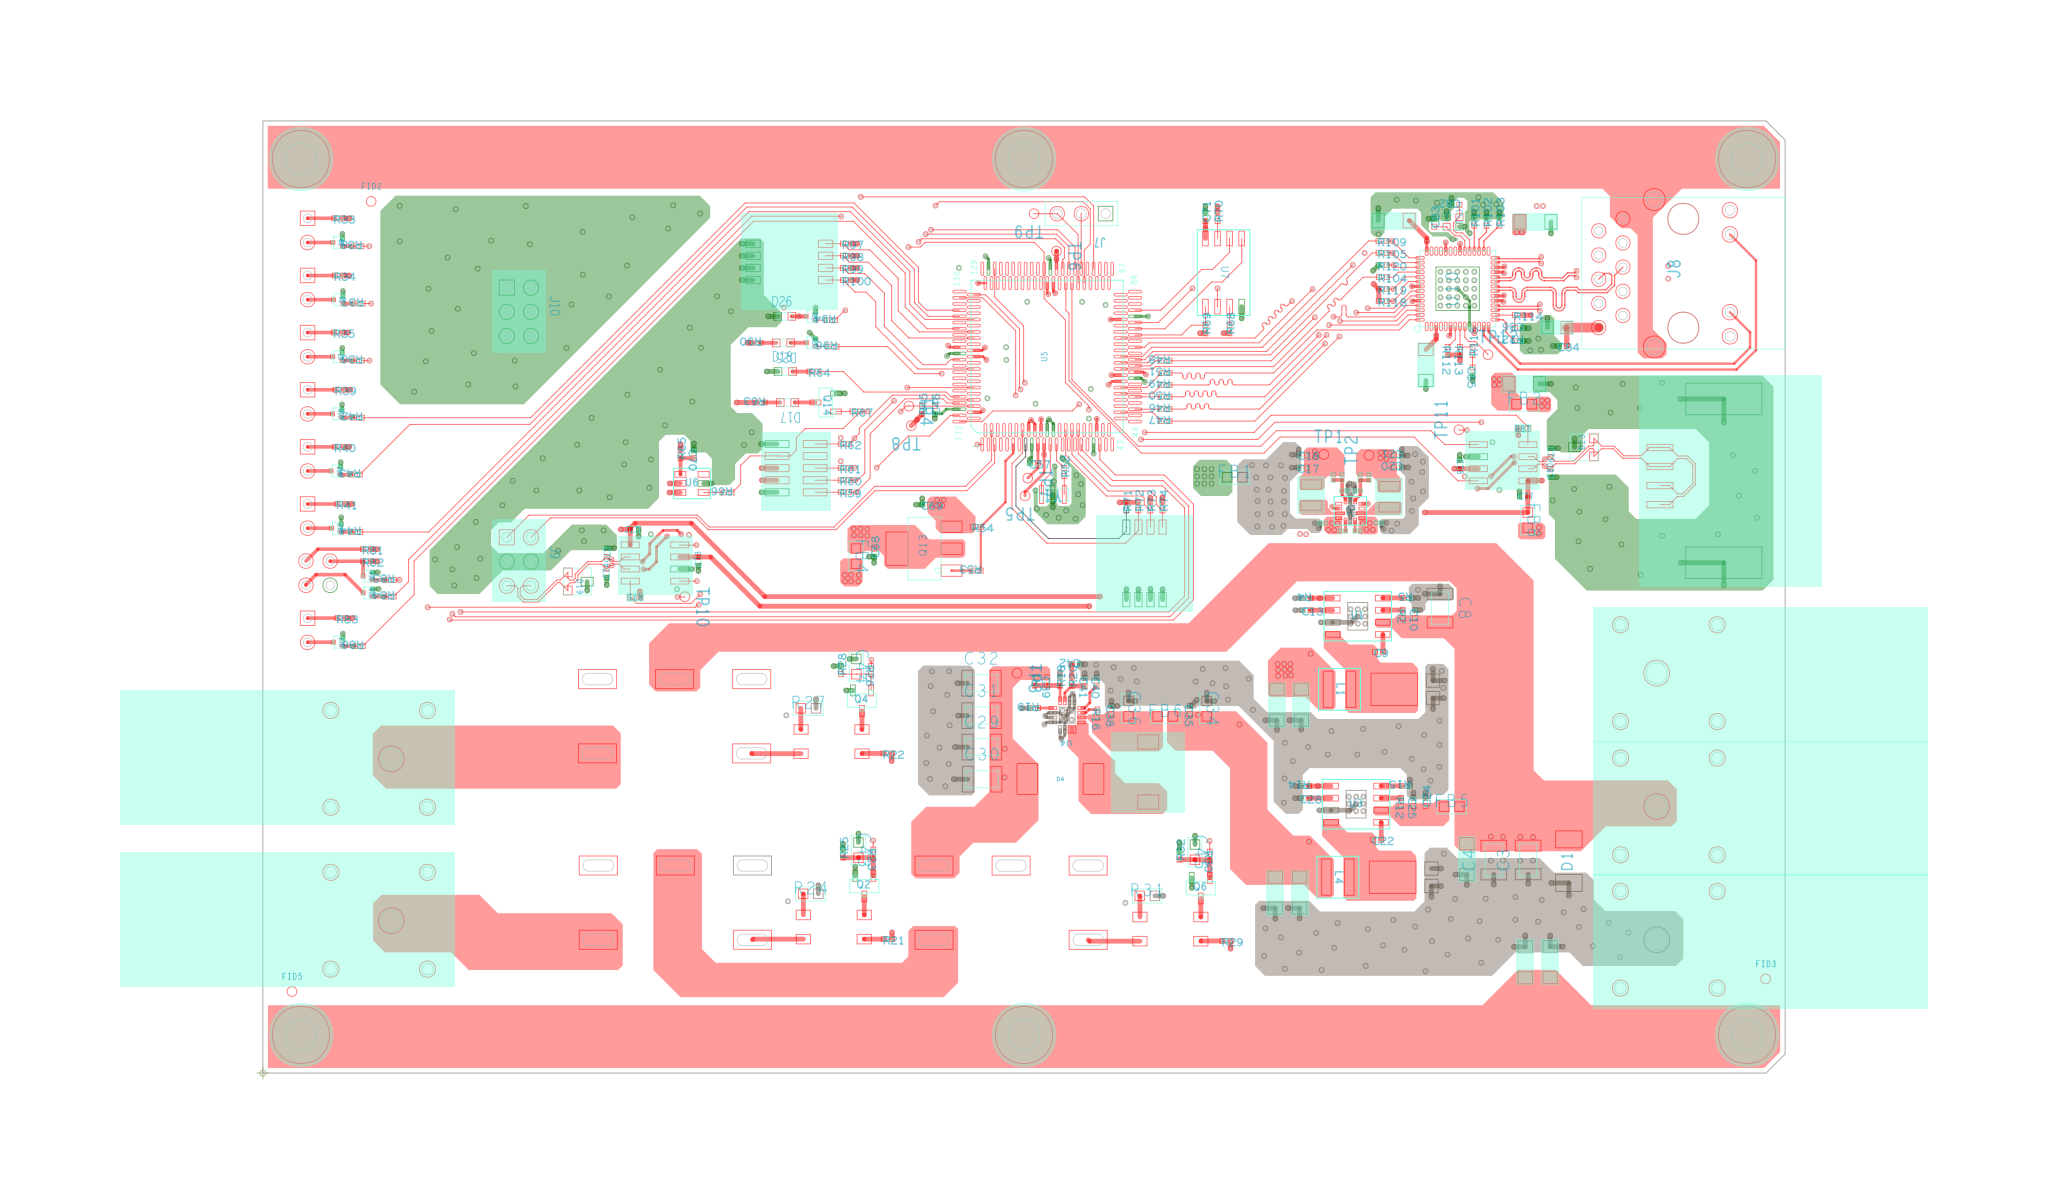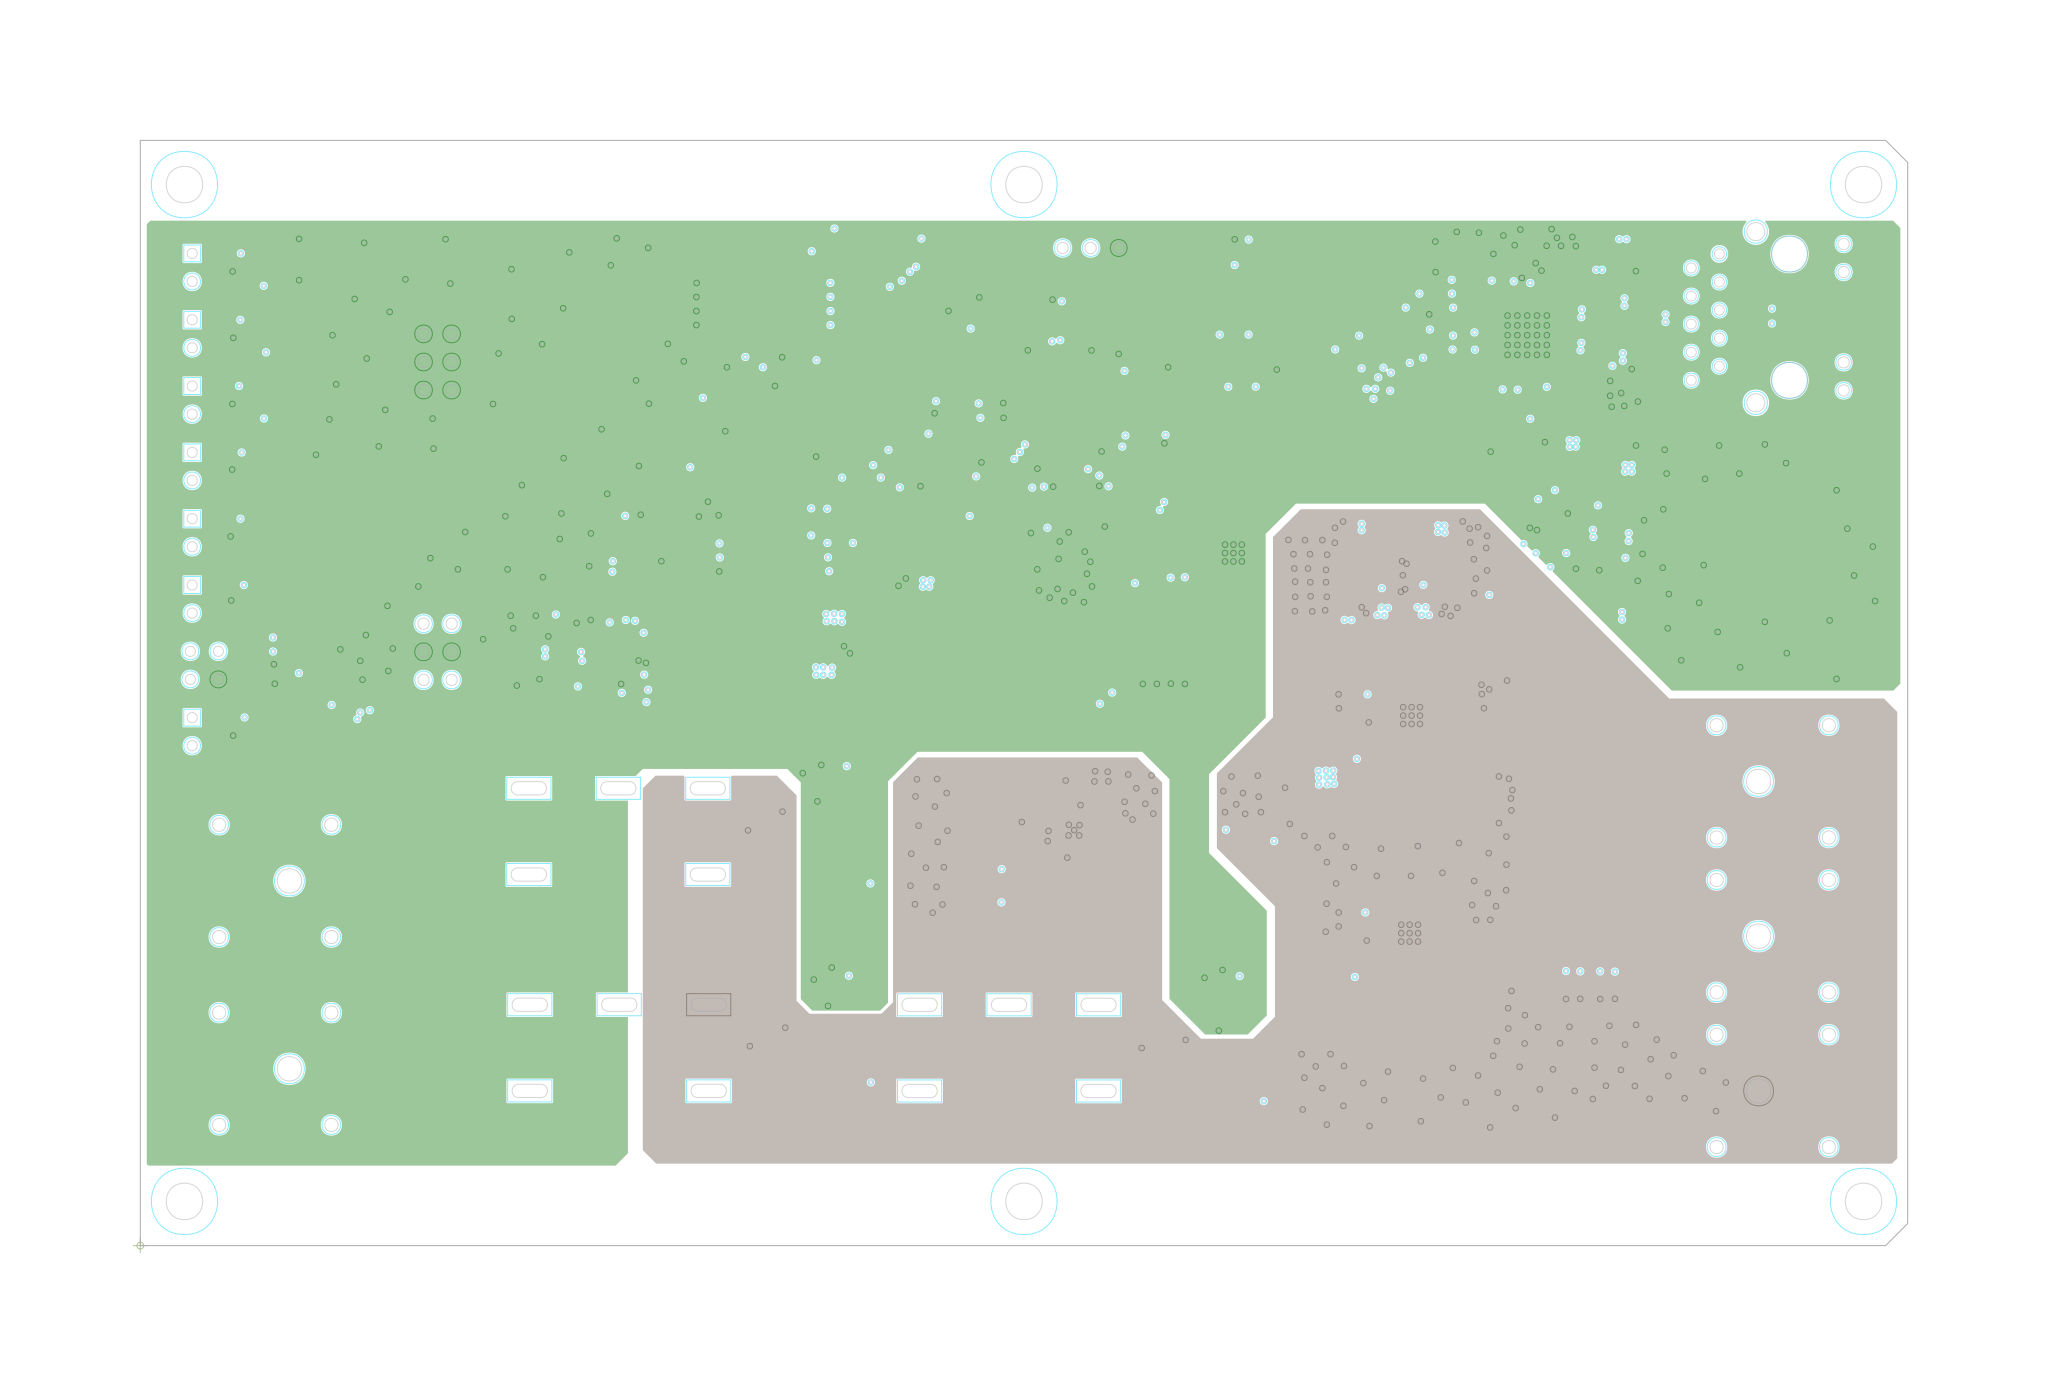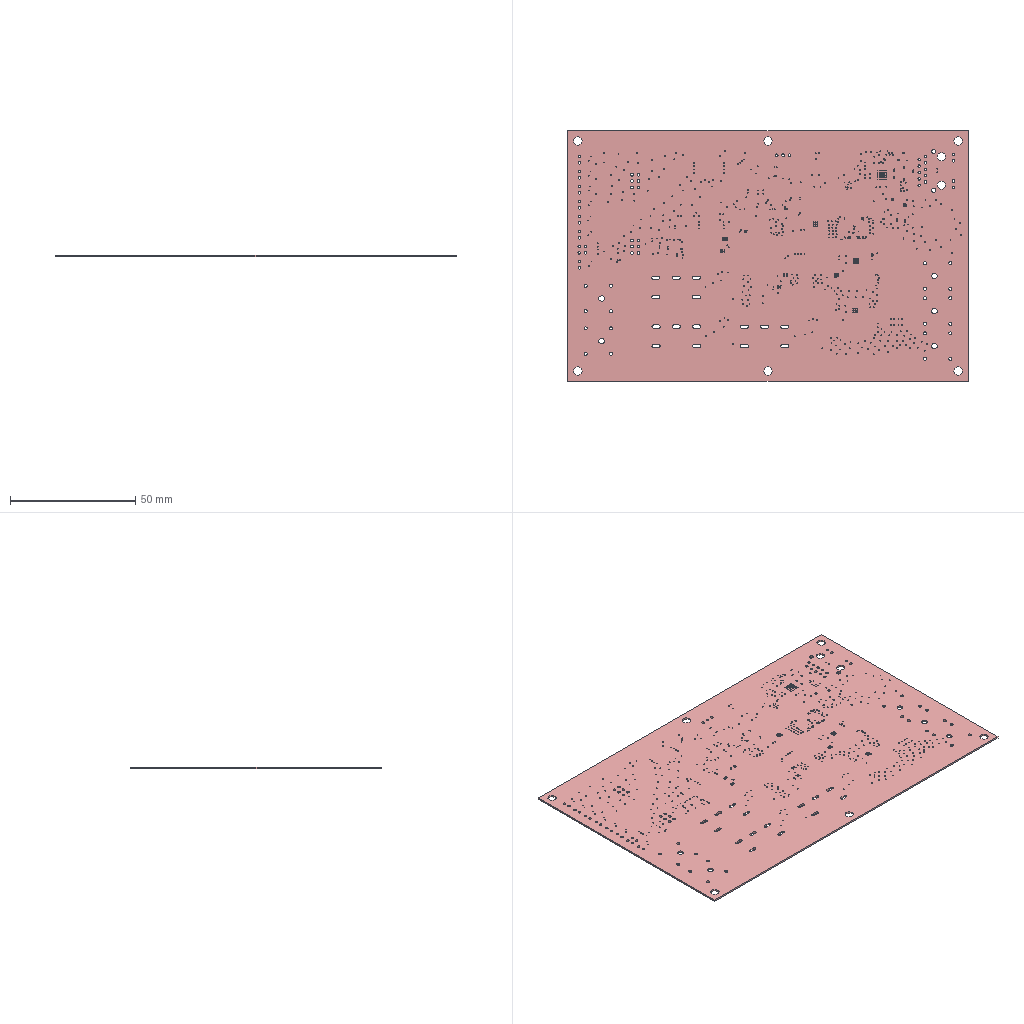Circuit board layout | Cadence Allegro | box 160 x 100 x 0.7 mm
Layer stack:
# Cadence Allegro layer stack of 2 (unit mm; from the constraint file cross-section; dielectric type: 0 not recorded (Allegro does not mark core vs prepreg), 3 surface material)
index,name,kind,layer,copper_thickness_mm,dielectric_type,dielectric_thickness_mm,dielectric_material,dielectric_constant
0,Top Surface,other,,,,,,
1,TOP,copper,TOP,0.0305,,,,
2,Dielectric1,dielectric,,,0,0.2032,FR-4,4.5
3,GND,copper,GND,0.0305,,,,
4,Dielectric2,dielectric,,,0,0.2032,FR-4,4.5
5,POWER,copper,POWER,0.0305,,,,
6,Dielectric3,dielectric,,,0,0.2032,FR-4,4.5
7,BOTTOM,copper,BOTTOM,0.0305,,,,
8,Bottom Surface,other,,,,,,
# drill layer pairs: low layer,high layer
drill_pair,TOP,BOTTOM
Part placement:
REFDES,COMP_VALUE,SYM_NAME,SYM_X,SYM_Y,SYM_ROTATE,SYM_MIRROR
C1,0.1uF,0402,5255.815,929.472,90.000,YES
C2,1nF,0402,5203.236,928.917,270.000,YES
C3,10uF_50V,1210,5236.091,881.236,90.000,NO
C4,10uF_50V,1210,5093.579,880.543,90.000,NO
C5,0.1uF,0402,5132.177,928.886,270.000,YES
C6,0.1uF,0402,5081.394,928.713,270.000,YES
C7,1nF_2kv,1206,5223.642,458.039,270.000,NO
C8,4.7uF_50V,1210,4871.276,1922.413,270.000,NO
C9,0.1uF,0402,4618.441,1741.791,0.000,NO
C10,0.1uF,0402,4768.024,1897.736,270.000,NO
C11,100uF_6.3V,1206,4196.335,1522.984,270.000,NO
C12,100uF_6.3V,1206,4296.965,1523.051,270.000,NO
C13,470pF,0402,4319.169,1913.894,0.000,NO
C14,4.7uF_6.3V,0201,4617.413,2275.484,180.000,NO
C15,4.7uF_6.3V,0201,4386.961,2273.791,0.000,NO
C16,10pF,0201,4431.000,2463.535,90.000,NO
C17,22uF_6.3V,0402,4302.398,2503.622,0.000,NO
C18,22uF_6.3V,0402,4303.248,2556.858,0.000,NO
C19,10pF,0201,4541.429,2462.433,90.000,NO
C20,10uF_6.3V,0402,4696.803,2504.610,180.000,NO
C21,10uF_6.3V,0402,4696.776,2553.764,180.000,NO
C22,0.1uF,0402,4611.441,964.791,0.000,NO
C23,10uF_50V,1206,4982.193,884.799,90.000,NO
C24,1uF,0402,4811.551,1120.925,90.000,NO
C25,0.1uF,0402,4761.024,1120.736,270.000,NO
C26,100uF_6.3V,1206,4289.965,746.051,270.000,NO
C27,100uF_6.3V,1206,4189.335,745.984,270.000,NO
C28,470pF,0402,4312.169,1136.894,0.000,NO
C29,4.7uF_50V,1210,2975.161,1347.945,0.000,NO
C30,4.7uF_50V,1210,2976.256,1215.130,0.000,NO
C31,4.7uF_50V,1210,2974.024,1478.004,0.000,NO
C32,4.7uF_50V,1210,2973.433,1612.031,0.000,NO
C33,10uF_50V,1206,2970.370,1340.913,180.000,YES
C34,10uF_16V,0603,3905.988,1506.535,270.000,NO
C35,0.1uF,0402,3836.575,1501.610,270.000,NO
C36,10uF_16V,0603,3582.047,1507.114,270.000,NO
C37,10uF_50V,1206,2970.870,1222.839,180.000,YES
C38,0.1uF,0402,3511.059,1501.157,270.000,NO
C39,20pF_25V,0402,3245.874,1619.213,270.000,NO
C40,47nF_10V,0402,3450.453,1618.110,270.000,NO
C41,100pF_16V,0402,3400.661,1617.000,270.000,NO
C42,0.1uF,0402,3364.358,1689.886,180.000,NO
C43,2.2nF_50V,0603,2464.520,921.850,270.000,NO
C44,2.2nF_50V,0603,2455.957,1680.697,270.000,NO
C45,2.2nF_50V,0603,3857.189,913.346,270.000,NO
C46,0.1uF,0402,2780.705,2741.437,90.000,NO
C47,10uF_10V,0603,3317.331,3188.803,0.000,YES
C48,0.1uF,0402,3254.417,3266.378,180.000,YES
C49,0.1uF,0402,3549.661,2869.283,270.000,YES
C50,0.1uF,0402,3217.000,2599.795,180.000,YES
C51,0.1uF,0402,3034.114,3001.382,0.000,YES
C52,0.1uF,0402,3236.941,2658.358,0.000,YES
C53,0.1uF,0402,3609.000,2882.224,270.000,YES
C54,0.1uF,0402,3267.819,3325.811,180.000,YES
C55,0.1uF,0402,2882.472,2985.067,270.000,YES
C56,10uF_10V,0603,2794.520,2984.303,270.000,YES
C57,0.22uF,0402,3190.701,2521.654,0.000,NO
C58,10uF_10V,0603,2925.579,3297.961,90.000,YES
C59,0.1uF,0402,3169.465,2751.110,90.000,YES
C60,0.1uF,0402,3033.862,2948.642,0.000,YES
C61,0.1uF,0402,2990.244,3282.819,90.000,YES
C62,0.1uF,0402,3547.087,3132.346,90.000,YES
C63,0.1uF,0402,3442.697,2846.890,180.000,YES
C64,0.1uF,0402,3486.980,3132.303,90.000,YES
C65,0.1uF,0402,3434.421,2658.268,180.000,YES
C66,0.1uF,0402,3211.118,3189.185,180.000,YES
C67,0.1uF,0402,2941.248,2748.118,90.000,YES
C68,2.2uF,0402,2529.287,2151.634,90.000,NO
C69,2.2uF,0402,2744.913,2350.260,0.000,NO
C70,NC,0402,1783.713,2559.197,270.000,NO
C71,0.1uF,0402,3900.539,3539.610,90.000,NO
C72,0.1uF/50V,C0402,1537.614,2249.240,180.000,NO
C73,0.1uF/50V,C0402,1802.283,2116.236,90.000,NO
C74,47pF/50V,C0402,1422.764,2066.839,90.000,NO
C75,47pF/50V,C0402,1422.772,2152.642,270.000,NO
C76,47nF/50V,C0402,1655.654,2196.618,180.000,YES
C77,0.1uF/50V,C0402,5217.319,2383.724,0.000,NO
C78,0.1uF/50V,C0402,4952.650,2516.728,270.000,NO
C79,47pF/50V,C0402,5328.169,2566.126,270.000,NO
C80,47pF/50V,C0402,5329.161,2481.323,90.000,NO
C81,47nF/50V,C0402,5099.280,2436.346,0.000,YES
C82,6pF_1%,0402,4935.124,3590.128,180.000,NO
C83,6pF_1%,0402,4846.808,3515.924,90.000,NO
C84,0.1uF,0402,5379.007,3006.491,0.000,NO
C85,47pF,0402,5006.083,2900.662,270.000,NO
C86,0.1uF,0402,5197.268,3080.205,180.000,NO
C87,0.1uF,0402,4814.862,3388.890,90.000,YES
C88,0.1uF,0402,4914.433,3103.504,270.000,YES
C89,0.1uF,0402,5082.740,3298.197,0.000,YES
C90,0.1uF,0402,5083.543,3232.583,0.000,YES
C91,0.1uF,0402,5013.547,3103.697,270.000,YES
C92,0.1uF,0402,4804.024,3252.988,180.000,YES
C93,0.1uF,0402,4805.969,3191.358,180.000,YES
C94,0.1uF,0402,4902.161,3388.575,90.000,YES
C95,0.1uF,0402,4953.748,3388.339,90.000,YES
C96,0.1uF,0402,5084.028,3182.937,0.000,YES
C97,0.1uF,0402,5083.260,3346.500,0.000,YES
C98,0.1uF,0402,4855.610,3104.161,270.000,YES
CB1,22uF_10V,0805,5355.680,3082.448,180.000,NO
CB2,22uF_10V,1206,4679.571,3525.020,180.000,NO
CB3,22uF_10V,1206,5266.339,3519.437,0.000,NO
CB4,22uF_10V,1206,5219.425,2850.093,0.000,NO
CB5,22uF_10V,1206,4812.812,2927.908,270.000,NO
D1,SMBJ33CA,DO-214AA,5404.406,876.315,90.000,NO
D2,PDS760-13,PDS760,4762.260,1586.618,0.000,NO
D3,PDS760-13,PDS760,4755.260,809.618,0.000,NO
D4,B540C-13-F,SMC,3300.154,1215.972,0.000,NO
D5,SMAJ16A,DO-214AC,2230.827,631.843,90.000,YES
D6,SMAJ16A,DO-214AC,1750.311,552.874,0.000,YES
D7,SMAJ16A,DO-214AC,2220.673,1400.406,90.000,YES
D8,SMAJ16A,DO-214AC,1740.748,1321.720,0.000,YES
D9,SMAJ16A,DO-214AC,3628.323,625.173,90.000,YES
D10,SMAJ16A,DO-214AC,3120.980,550.370,0.000,YES
D11,MHK1375CGBTD,LED-TH_MHK1375CRBTD,185.043,3484.280,270.000,NO
D12,MHK1375CGBTD,LED-TH_MHK1375CRBTD,185.043,3248.059,270.000,NO
D13,MHK1375CGBTD,LED-TH_MHK1375CRBTD,185.043,3011.839,270.000,NO
D14,MHK1375CRBTD,LED-TH_MHK1375CRBTD,185.043,2775.618,270.000,NO
D15,MHK1375CRBTD,LED-TH_MHK1375CRBTD,185.043,2539.398,270.000,NO
D16,MHK1375CRBTD,LED-TH_MHK1375CRBTD,185.043,2303.177,270.000,NO
D17,XL-TD1608SURC,LED0603,2170.984,2772.713,180.000,NO
D18,XL-TD1608SYGC,LED0603,2161.807,2900.945,0.000,NO
D19,SM24CANA-02HTG,SOT23-3,1262.067,2070.106,270.000,NO
D20,CSD87502Q2,DFN-6_2X2,1634.961,2108.839,90.000,YES
D21,MHK2396YGBTD,LED_D3_WX2,228.350,2066.957,270.000,NO
D22,MHK1375CGBTD,LED-TH_MHK1375CRBTD,185.039,1830.709,270.000,NO
D23,SM24CANA-02HTG,SOT23-3,5508.000,2549.929,90.000,NO
D24,CSD87502Q2,DFN-6_2X2,5119.972,2524.126,270.000,YES
D25,XL-TD1608SYGC,LED0603,2154.189,3019.417,180.000,NO
D26,XL-TD1608SURC,LED0603,2159.248,3128.795,0.000,NO
FB1,BLM18KG300TN1D,0603,4022.043,2463.720,0.000,NO
FB2,BLM18KG300TN1D,0603,5219.364,2765.824,0.000,NO
FB3,BLM18KG300TN1D,0603,5234.535,3520.157,180.000,YES
FB4,BLM18KG300TN1D,0603,2454.500,2137.295,270.000,NO
FB5,BLM18KG300TN1D,0603,4919.642,1101.654,0.000,NO
FB6,BLM18KG300TN1D,0603,3734.146,1474.689,0.000,NO
FB7,BLM18KG300TN1D,0603,4367.000,2183.000,0.000,YES
FB8,BLM18KG300TN1D,0603,5234.536,2286.306,270.000,NO
FID1,FIDUCIAL_1MM,MARK40,6218.539,389.295,0.000,YES
FID2,FIDUCIAL_1MM,MARK40,447.854,3604.295,0.000,NO
FID3,FIDUCIAL_1MM,MARK40,6218.657,389.295,0.000,NO
FID4,FIDUCIAL_1MM,MARK40,447.953,3604.295,0.000,YES
FID5,FIDUCIAL_1MM,MARK40,120.244,337.295,0.000,NO
FID6,FIDUCIAL_1MM,MARK40,120.559,337.295,0.000,YES
J1,24.245.2,C7437326,5767.717,1102.362,180.000,NO
J2,24.245.1,C7437326,5767.717,551.181,180.000,NO
J3,24.245.1,C7437326,531.496,1299.213,0.000,NO
J4,24.245.2,C7437326,531.496,629.921,0.000,NO
J5,24.245.1,C7437326,5767.717,1653.543,180.000,NO
J6,Header_JTAG_2x5_1P27mm,JTAG_2X5_1P27MM,2206.571,2501.346,90.000,NO
J7,header_2.54_3,HDR_1X3,3487.157,3553.693,180.000,NO
J8,HR915330AE,HR915330AE,5877.953,3307.087,90.000,NO
J9,A2541WR-2x3P,DIP_2X3_254MM,1059.606,2115.150,270.000,NO
J10,A2541WR-2x3P,DIP_2X3_254MM,1059.606,3147.606,270.000,NO
J11,349128040,349128040,5913.386,2448.819,90.000,NO
L1,FEXL0430A-2R2M,L_41X41_H210_BOURNS,4455.374,1586.843,270.000,NO
L2,DFE252012PD-R47M,1008,4338.772,2389.969,90.000,NO
L3,DFE252012PD-R47M,1008,4661.961,2383.071,90.000,NO
L4,FEXL0430A-2R2M,L_41X41_H210_BOURNS,4448.374,809.843,270.000,NO
L5,SLF7045T100M,SMD_7X7,3663.744,1245.185,270.000,NO
MH1,MOUNTING_HOLE,HOLE3_3MM_6,6141.732,3779.528,0.000,NO
MH2,MOUNTING_HOLE,HOLE3_3MM_6,157.480,3779.528,0.000,NO
MH3,MOUNTING_HOLE,HOLE3_3MM_6,157.480,157.480,0.000,NO
MH4,MOUNTING_HOLE,HOLE3_3MM_6,6141.732,157.480,0.000,NO
MH5,MOUNTING_HOLE,HOLE3_3MM_6,3149.606,157.480,0.000,NO
MH6,MOUNTING_HOLE,HOLE3_3MM_6,3149.606,3779.528,0.000,NO
Q1,TLP187,TLP187,2362.610,603.874,90.000,NO
Q2,BSS138,003_SOT23B,2526.213,815.496,270.000,NO
Q3,TLP187,TLP187,2353.047,1370.720,90.000,NO
Q4,BSS138,003_SOT23B,2516.650,1582.343,270.000,NO
Q5,TLP187,TLP187,3755.280,595.370,90.000,NO
Q6,BSS138,003_SOT23B,3918.882,806.992,270.000,NO
Q7,CJ3134K KF,SOT-723,308.504,2962.004,90.000,NO
Q8,CJ3134K KF,SOT-723,311.874,3197.748,90.000,NO
Q9,CJ3134K KF,SOT-723,309.358,3434.394,90.000,NO
Q10,CJ3134K KF,SOT-723,307.776,2725.854,90.000,NO
Q11,CJ3134K KF,SOT-723,302.209,2489.756,90.000,NO
Q12,CJ3134K KF,SOT-723,304.539,2253.000,90.000,NO
Q13,BCP56-16TX,BCP56_SOT-223,2737.874,2168.087,90.000,NO
Q14,BSS138,003_SOT23B,2371.516,2735.583,180.000,NO
Q15,CJ3134K KF,SOT723,1729.902,2089.772,0.000,YES
Q16,CJ3134K KF,SOT-723,434.465,2054.969,90.000,NO
Q17,CJ3134K KF,SOT-723,311.413,1781.638,90.000,NO
Q18,CJ3134K KF,SOT-723,434.886,1985.878,90.000,NO
Q19,CJ3134K KF,SOT723,5025.031,2543.193,180.000,YES
Q20,CJ3134K KF,SOT-723,2268.819,3019.654,90.000,NO
Q21,CJ3134K KF,SOT-723,2267.772,3128.799,90.000,NO
R1,1M,1206,5326.661,459.004,90.000,NO
R2,100K,0402,4717.106,1897.874,270.000,NO
R3,51K,0402,4336.000,1947.000,270.000,YES
R4,15K,0402,4319.480,1963.724,180.000,NO
R5,20K,0402,4737.150,1964.650,180.000,NO
R6,68K,0201,4465.665,2463.618,270.000,NO
R7,100k,0201,4469.134,2241.382,0.000,NO
R8,102K,0201,4477.224,2407.067,0.000,NO
R9,100k,0201,4530.858,2241.882,180.000,NO
R10,220K,0201,4576.213,2462.854,270.000,NO
R11,110K,0201,4530.205,2406.669,180.000,NO
R12,100K,0402,4710.106,1120.874,270.000,NO
R13,51.1K,0402,4329.000,1170.000,270.000,YES
R14,9.09K,0402,4312.480,1186.724,180.000,NO
R15,20K,0402,4730.150,1187.650,180.000,NO
R16,10K,0402,3452.902,1486.622,270.000,NO
R17,88.7K_1%,0402,3193.323,1618.815,90.000,NO
R18,10K,0402,3298.213,1618.319,90.000,NO
R19,78.7K_1%,0402,3191.150,1508.945,180.000,NO
R20,2.55K_1%,0402,3347.547,1617.744,90.000,NO
R21,470R,0402,2587.181,553.748,0.000,NO
R22,470R,0402,2585.618,1321.594,0.000,NO
R23,100R,0402,2525.567,907.496,270.000,NO
R24,2k_0603,0603,2267.039,741.295,0.000,NO
R25,4.7K,0402,2400.362,907.484,90.000,NO
R26,100R,0402,2517.004,1666.343,270.000,NO
R27,2k_0603,0603,2257.476,1508.142,0.000,NO
R28,4.7K,0402,2391.799,1666.331,90.000,NO
R29,470R,0402,3987.850,546.244,0.000,NO
R30,100R,0402,3918.236,898.992,270.000,NO
R31,2k_0603,0603,3659.709,732.791,0.000,NO
R32,4.7K,0402,3793.031,898.980,90.000,NO
R33,1.8K,0402,312.862,3534.524,0.000,NO
R34,1.8K,0402,314.287,3297.642,0.000,NO
R35,1.8K,0402,311.543,3062.012,0.000,NO
R36,100R,0402,393.079,2946.142,180.000,NO
R37,100R,0402,396.000,3182.000,180.000,NO
R38,100R,0402,391.000,3419.000,180.000,NO
R39,1.8K,0402,318.150,2825.307,0.000,NO
R40,1.8K,0402,315.472,2589.228,0.000,NO
R41,1.8K,0402,324.000,2353.000,0.000,NO
R42,100R,0402,393.000,2710.000,180.000,NO
R43,100R,0402,384.555,2474.642,180.000,NO
R44,100R,0402,386.209,2237.201,180.000,NO
R45,4.7K,0402,2727.941,2741.709,90.000,NO
R46,33R,0402,3734.963,2745.396,180.000,NO
R47,33R,0402,3734.963,2695.937,180.000,NO
R48,33R,0402,3734.963,2945.331,180.000,NO
R49,33R,0402,3734.963,2845.303,180.000,NO
R50,33R,0402,3734.963,2796.508,180.000,NO
R51,33R,0402,3734.963,2894.827,180.000,NO
R52,0R,0402,3316.000,2485.000,90.000,NO
R53,10K,0402,2953.559,2077.638,180.000,NO
R54,2.2K,0402,2954.378,2258.654,0.000,NO
R55,4.7K,0402,2407.980,2402.504,0.000,YES
R56,4.7K,0402,2408.130,2451.764,0.000,YES
R57,4.7K,0402,2407.795,2502.161,0.000,YES
R58,4.7K,0402,2407.772,2601.169,0.000,YES
R59,33R,0402,2408.016,2402.177,0.000,NO
R60,33R,0402,2408.051,2451.764,0.000,NO
R61,33R,0402,2407.961,2502.008,0.000,NO
R62,33R,0402,2408.185,2601.177,0.000,NO
R63,5.6K,0402,2059.602,2772.598,180.000,NO
R64,1.8K,0402,2278.717,2900.602,0.000,NO
R65,100K,0402,1728.303,2559.047,90.000,NO
R66,0R,0402,1923.098,2400.669,180.000,NO
R67,100R,0402,2456.091,2735.732,0.000,NO
R68,4.7K,0402,4000.000,3076.000,90.000,NO
R69,4.7K,0402,3900.598,3075.724,90.000,NO
R70,10K,0402,3950.524,3539.591,90.000,NO
R71,4.7K,0402,3573.228,2343.252,90.000,NO
R72,4.7K,0402,3622.520,2343.551,90.000,NO
R73,4.7K,0402,3672.319,2342.890,90.000,NO
R74,4.7K,0402,3722.744,2343.075,90.000,NO
R75,4.7K/1%,R0402,1540.157,1968.398,180.000,NO
R76,60R,R0402,1518.346,2084.146,180.000,YES
R77,60R,R0402,1517.823,2134.346,180.000,YES
R78,10K,0402,1746.965,2147.276,180.000,YES
R79,100R,0402,1746.965,1952.417,270.000,YES
R80,100R,0402,1730.161,2024.906,0.000,YES
R81,1.8K,0402,431.102,2166.181,0.000,NO
R82,1.8K,0402,431.260,2116.256,0.000,NO
R83,1.8K,0402,324.976,1881.390,0.000,NO
R84,100R,0402,524.720,1970.390,180.000,NO
R85,100R,0402,525.051,2039.295,180.000,NO
R86,100R,0402,396.575,1765.335,180.000,NO
R87,4.7K/1%,R0402,5214.776,2664.567,0.000,NO
R88,60R,R0402,5236.587,2548.819,0.000,YES
R89,60R,R0402,5237.110,2498.618,0.000,YES
R90,1.8K,0402,2042.984,3019.764,180.000,NO
R91,1.8K,0402,2173.000,3129.000,0.000,YES
R92,10K,0402,5009.000,2482.791,0.000,YES
R93,100R,0402,5025.516,2658.929,0.000,YES
R94,100R,0402,2350.783,3113.307,180.000,NO
R95,100R,0402,5025.772,2608.059,180.000,YES
R96,100R,0402,2357.091,3004.031,180.000,NO
R97,4.7K,0402,2417.512,3429.559,0.000,NO
R98,4.7K,0402,2417.039,3379.571,0.000,NO
R99,4.7K,0402,2416.724,3328.957,0.000,NO
R100,4.7K,0402,2417.402,3278.980,0.000,NO
R101,49R9,0402,5012.327,3520.984,90.000,NO
R102,49R9,0402,5063.728,3520.496,90.000,NO
R103,4.99K,0402,5116.386,3520.724,90.000,NO
R104,33R,0402,4634.745,3290.982,0.000,NO
R105,33R,0402,4633.659,3391.112,0.000,NO
R106,33R,0402,4633.955,3341.214,180.000,YES
R107,33R,0402,4634.223,3241.276,180.000,YES
R108,33R,0402,4634.339,3192.212,180.000,YES
R109,33R,0402,4633.151,3440.765,0.000,NO
R110,510R,0402,5884.886,3284.606,180.000,YES
R111,510R,0402,5884.680,3337.640,180.000,YES
R112,4.7K,0402,4902.905,2985.637,270.000,NO
R113,4.7K,0402,4953.783,2985.834,270.000,NO
R114,4.7K,0402,5197.189,3133.866,0.000,NO
R115,49R9,0402,5005.780,2985.543,90.000,NO
R116,4.7K,0402,4633.116,3440.580,180.000,YES
R117,4.7K,0402,4633.769,3391.057,180.000,YES
R118,4.7K,0402,4634.339,3192.215,0.000,NO
R119,4.7K,0402,4634.326,3241.666,0.000,NO
R120,4.7K,0402,4633.962,3341.033,0.000,NO
R121,4.7K,0402,5197.244,3027.252,180.000,NO
RY1,HFV9-012-1ZR,HFV9-012-1ZR,1707.008,704.669,0.000,NO
RY2,HFV9-012-1ZR,HFV9-012-1ZR,1703.760,1475.472,0.000,NO
RY3,HFV9-012-1ZR,HFV9-012-1ZR,3096.366,704.354,0.000,NO
S1,DSHP04TS-S,DSHP04TS-S,3648.122,2107.520,0.000,NO
S2,DSHP04TS-S,DSHP04TS-S,2178.780,3354.071,270.000,NO
TP1,TP,S0400CI,4390.276,2557.839,0.000,NO
TP2,TP,S0400CI,4577.488,2553.984,90.000,NO
TP3,TP,S0400CI,3120.697,1653.559,270.000,NO
TP4,TP,S0400CI,2673.000,2758.000,270.000,NO
TP5,TP,S0400CI,3154.000,2387.000,180.000,NO
TP6,TP,S0400CI,3284.098,3398.539,270.000,NO
TP7,TP,S0400CI,3165.000,2460.000,270.000,NO
TP8,TP,S0400CI,2683.000,2677.000,180.000,NO
TP9,TP,S0400CI,3191.134,3553.587,180.000,NO
TP10,TP,S0400CI,1746.307,1969.622,270.000,NO
TP11,TP,S0400CI,4949.626,2660.343,90.000,NO
TP12,TP,S0400CI,5069.501,2970.197,0.000,NO
U1,LMR14050SQDDARQ1,SOP8P_60_PAD29X21_127_H170,4530.713,1888.748,0.000,NO
U2,TPS62442,QFN14P_27X23_05_H100,4499.909,2324.362,270.000,NO
U3,LMR14050SQDDARQ1,SOP8P_60_PAD29X21_127_H170,4523.713,1111.748,0.000,NO
U4,TPS55340RTER,WQFN16-3X3,3387.500,1539.012,180.000,NO
U5,S32K314EHTVBPBST_MaxQFP172,MQFP172_0P65_16X16,3245.720,2962.535,90.000,NO
U6,TPS3808G33DBV,SOT23_6P_29X28_H150,1775.752,2437.972,0.000,NO
U7,W25Q128JVSIQ,SO8P_79_127_H220,3975.512,3310.016,270.000,NO
U8,TJA1462AT,SO8,1622.630,2109.138,90.000,NO
U9,TJA1462AT,SO8,5132.303,2523.827,270.000,NO
U10,88EA1512_QFN56,QFN50P800X800X100-56N_180X180EP,4944.134,3242.980,90.000,NO
Y1,CSTNE16M0V53C000R0,CSTNE16M0V53C000R0,3269.055,2392.740,180.000,NO
Y2,XRCGB25M000F3A00R00,CRYSTAL_SM,4924.941,3519.299,0.000,NO
Pad and via stacks, first 111 of 413 lines:
# Allegro (Cadence) via spans and padstacks; design units: ("mils" 3 1000)
# via spans: padstack,start_layer,end_layer,net_example,count
VIA12X20,ETCH/TOP,ETCH/BOTTOM,GND,686
# Allegro padstack definitions: name,start_layer,end_layer,drill,plating,holeType,type
PAD19,"ETCH/TOP","ETCH/TOP",0.0,"NON_PLATED","none","smd"
PAD13,"ETCH/TOP","ETCH/TOP",0.0,"NON_PLATED","none","smd"
PAD12,"ETCH/TOP","ETCH/TOP",0.0,"NON_PLATED","none","smd"
PAD17,"ETCH/TOP","ETCH/TOP",0.0,"NON_PLATED","none","smd"
PAD15,"ETCH/TOP","ETCH/TOP",0.0,"NON_PLATED","none","smd"
PAD16,"ETCH/TOP","ETCH/TOP",0.0,"NON_PLATED","none","smd"
PAD1,"ETCH/TOP","ETCH/TOP",0.0,"NON_PLATED","none","smd"
PAD46,"ETCH/TOP","ETCH/TOP",0.0,"NON_PLATED","none","smd"
PAD44,"ETCH/TOP","ETCH/TOP",0.0,"NON_PLATED","none","smd"
PAD8,"ETCH/TOP","ETCH/TOP",0.0,"NON_PLATED","none","smd"
PAD5,"ETCH/TOP","ETCH/TOP",0.0,"NON_PLATED","none","smd"
PAD9,"ETCH/TOP","ETCH/TOP",0.0,"NON_PLATED","none","smd"
PAD10,"ETCH/TOP","ETCH/TOP",0.0,"NON_PLATED","none","smd"
PAD25,"ETCH/TOP","ETCH/TOP",0.0,"NON_PLATED","none","smd"
PAD4,"ETCH/TOP","ETCH/TOP",0.0,"NON_PLATED","none","smd"
PAD7,"ETCH/TOP","ETCH/TOP",0.0,"NON_PLATED","none","smd"
PAD6,"ETCH/TOP","ETCH/TOP",0.0,"NON_PLATED","none","smd"
PAD3,"ETCH/TOP","ETCH/TOP",0.0,"NON_PLATED","none","smd"
PAD31,"ETCH/TOP","ETCH/TOP",0.0,"NON_PLATED","none","smd"
PAD22,"ETCH/TOP","ETCH/TOP",0.0,"NON_PLATED","none","smd"
PAD41,"ETCH/TOP","ETCH/TOP",0.0,"NON_PLATED","none","smd"
PAD42,"ETCH/TOP","ETCH/TOP",0.0,"NON_PLATED","none","smd"
PAD43,"ETCH/TOP","ETCH/TOP",0.0,"NON_PLATED","none","smd"
PAD45,"ETCH/TOP","ETCH/TOP",0.0,"NON_PLATED","none","smd"
PAD2,"ETCH/TOP","ETCH/TOP",0.0,"NON_PLATED","none","smd"
PAD14,"ETCH/TOP","ETCH/TOP",0.0,"NON_PLATED","none","smd"
PAD21,"ETCH/TOP","ETCH/TOP",0.0,"NON_PLATED","none","smd"
PAD28,"ETCH/TOP","ETCH/TOP",0.0,"NON_PLATED","none","smd"
PAD26,"ETCH/TOP","ETCH/TOP",0.0,"NON_PLATED","none","smd"
PAD27,"ETCH/TOP","ETCH/TOP",0.0,"NON_PLATED","none","smd"
PAD18,"ETCH/TOP","ETCH/TOP",0.0,"NON_PLATED","none","smd"
PAD29,"ETCH/TOP","ETCH/TOP",0.0,"NON_PLATED","none","smd"
PAD20,"ETCH/TOP","ETCH/TOP",0.0,"NON_PLATED","none","smd"
PAD39,"ETCH/TOP","ETCH/TOP",0.0,"NON_PLATED","none","smd"
PAD40,"ETCH/TOP","ETCH/TOP",0.0,"NON_PLATED","none","smd"
PAD30,"ETCH/TOP","ETCH/TOP",0.0,"NON_PLATED","none","smd"
PAD48,"ETCH/TOP","ETCH/TOP",0.0,"NON_PLATED","none","smd"
PAD47,"ETCH/TOP","ETCH/TOP",0.0,"NON_PLATED","none","smd"
PAD49,"ETCH/TOP","ETCH/TOP",0.0,"NON_PLATED","none","smd"
PAD50,"ETCH/TOP","ETCH/TOP",0.0,"NON_PLATED","none","smd"
PAD53,"ETCH/TOP","ETCH/TOP",0.0,"NON_PLATED","none","smd"
F45,"ETCH/TOP","ETCH/TOP",0.0,"NON_PLATED","none","smd"
R88X76,"ETCH/TOP","ETCH/TOP",0.0,"PLATED","none","smd"
R127X121,"ETCH/TOP","ETCH/TOP",0.0,"PLATED","none","smd"
R127X152,"ETCH/TOP","ETCH/TOP",0.0,"NON_PLATED","none","smd"
R14X25,"ETCH/TOP","ETCH/TOP",0.0,"NON_PLATED","none","smd"
R165X317,"ETCH/TOP","ETCH/TOP",0.0,"NON_PLATED","none","smd"
R259X218,"ETCH/TOP","ETCH/TOP",0.0,"NON_PLATED","none","smd"
R70X22,"ETCH/TOP","ETCH/TOP",0.0,"NON_PLATED","none","smd"
R75X85,"ETCH/TOP","ETCH/TOP",0.0,"NON_PLATED","none","smd"
Y5,"ETCH/TOP","ETCH/TOP",0.0,"NON_PLATED","none","smd"
R16X30,"ETCH/TOP","ETCH/TOP",0.0,"NON_PLATED","none","smd"
F62X58,"ETCH/TOP","ETCH/TOP",0.0,"PLATED","none","smd"
R15X28,"ETCH/TOP","ETCH/TOP",0.0,"NON_PLATED","none","smd"
R195X280,"ETCH/TOP","ETCH/TOP",0.0,"NON_PLATED","none","smd"
R45X200,"ETCH/TOP","ETCH/TOP",0.0,"NON_PLATED","none","smd"
R50X30,"ETCH/TOP","ETCH/TOP",0.0,"NON_PLATED","none","smd"
R127X120,"ETCH/TOP","ETCH/TOP",0.0,"NON_PLATED","none","smd"
R31X24,"ETCH/TOP","ETCH/TOP",0.0,"NON_PLATED","none","smd"
R215X60,"ETCH/TOP","ETCH/TOP",0.0,"NON_PLATED","none","smd"
S17,"ETCH/TOP","ETCH/TOP",0.0,"NON_PLATED","none","smd"
R23X25,"ETCH/TOP","ETCH/TOP",0.0,"NON_PLATED","none","smd"
R19X32,"ETCH/TOP","ETCH/TOP",0.0,"NON_PLATED","none","smd"
R61X15,"ETCH/TOP","ETCH/TOP",0.0,"NON_PLATED","none","smd"
R45X150,"ETCH/TOP","ETCH/TOP",0.0,"NON_PLATED","none","smd"
R12X8,"ETCH/TOP","ETCH/TOP",0.0,"NON_PLATED","none","smd"
R91X127,"ETCH/TOP","ETCH/TOP",0.0,"NON_PLATED","none","smd"
S91,"ETCH/TOP","ETCH/TOP",0.0,"NON_PLATED","none","smd"
R55X99,"ETCH/TOP","ETCH/TOP",0.0,"NON_PLATED","none","smd"
R299X199,"ETCH/TOP","ETCH/TOP",0.0,"NON_PLATED","none","smd"
R114X165,"ETCH/TOP","ETCH/TOP",0.0,"NON_PLATED","none","smd"
R60X90,"ETCH/TOP","ETCH/TOP",0.0,"NON_PLATED","none","smd"
R6X10,"ETCH/TOP","ETCH/TOP",0.0,"NON_PLATED","none","smd"
Y10,"ETCH/TOP","ETCH/TOP",0.0,"NON_PLATED","none","smd"
R114X74,"ETCH/TOP","ETCH/TOP",0.0,"NON_PLATED","none","smd"
R30X130,"ETCH/TOP","ETCH/TOP",0.0,"PLATED","none","smd"
R50X127,"ETCH/TOP","ETCH/TOP",0.0,"NON_PLATED","none","smd"
R18X20,"ETCH/TOP","ETCH/TOP",0.0,"NON_PLATED","none","smd"
R60X71,"ETCH/TOP","ETCH/TOP",0.0,"NON_PLATED","none","smd"
R48X71,"ETCH/TOP","ETCH/TOP",0.0,"NON_PLATED","none","smd"
R80X30,"ETCH/TOP","ETCH/TOP",0.0,"PLATED","none","smd"
FLASH_0,"ETCH/TOP","ETCH/TOP",0.0,"PLATED","none","smd"
Y3,"ETCH/TOP","ETCH/TOP",0.0,"PLATED","none","smd"
R170X25,"ETCH/TOP","ETCH/TOP",0.0,"PLATED","none","smd"
R70X25,"ETCH/TOP","ETCH/TOP",0.0,"PLATED","none","smd"
R43X14,"ETCH/TOP","ETCH/TOP",0.0,"PLATED","none","smd"
R33X10,"ETCH/TOP","ETCH/TOP",0.0,"PLATED","none","smd"
R636X23,"ETCH/TOP","ETCH/TOP",0.0,"PLATED","none","smd"
R155X35,"ETCH/TOP","ETCH/TOP",0.0,"PLATED","none","smd"
R60X20,"ETCH/TOP","ETCH/TOP",0.0,"PLATED","none","smd"
R120X70,"ETCH/TOP","ETCH/TOP",0.0,"PLATED","none","smd"
SMD0_45R,"ETCH/TOP","ETCH/TOP",0.0,"PLATED","none","smd"
Y42,"ETCH/TOP","ETCH/TOP",0.0,"PLATED","none","smd"
R85X65,"ETCH/TOP","ETCH/TOP",0.0,"PLATED","none","smd"
Y30,"ETCH/TOP","ETCH/TOP",0.0,"PLATED","none","smd"
R53X20,"ETCH/TOP","ETCH/TOP",0.0,"PLATED","none","smd"
R55X40,"ETCH/TOP","ETCH/TOP",0.0,"PLATED","none","smd"
R155X25,"ETCH/TOP","ETCH/TOP",0.0,"PLATED","none","smd"
F17X17,"ETCH/TOP","ETCH/TOP",0.0,"PLATED","none","smd"
F89X32,"ETCH/TOP","ETCH/TOP",0.0,"PLATED","none","smd"
R8X2,"ETCH/TOP","ETCH/TOP",0.0,"PLATED","none","smd"
SMD40X20,"ETCH/TOP","ETCH/TOP",0.0,"PLATED","none","smd"
R340X185,"ETCH/TOP","ETCH/TOP",0.0,"PLATED","none","smd"
R27X10,"ETCH/TOP","ETCH/TOP",0.0,"PLATED","none","smd"
R22X11,"ETCH/TOP","ETCH/TOP",0.0,"PLATED","none","smd"
R32X36,"ETCH/TOP","ETCH/TOP",0.0,"PLATED","none","smd"
S21X20,"ETCH/TOP","ETCH/TOP",0.0,"PLATED","none","smd"
Design rules, without the lines most boards share, first 12 of 34 lines:
# Cadence Allegro design rules of 2 (from the Constraint Manager export 2-constraints.dcfx, design unit mil; typed fields in mm)
# columns: name | kind | enabled | priority | scope1 | scope2 | descriptor | typed fields (field=value)
# Allegro precedence (priority 1 wins): 1 Region class-to-class, 2 Region class, 3 Region, 4 class-to-class, 5 DiffPair/Bus/NetGroup override, 6 NetClass, 7 constraint set (CSet) default
# per-layer values are written LAYER=value in the descriptor and LAYER:mm in the typed field; a maximum of 0 means no limit set
# --- net classes (and buses / net groups) ---
PHY_TX | NetClass | enabled | 6 | 1512_MII_TX_CTRL_PTD11, 1512_MII_TXD3_PTD5, 1512_MII_TXD2_PTD6, 1512_MII_TXD1_PTB4, 1512_MII_TXD0_PTB5, 1512_MII_TX_CLK_PTC0 | All | Net Class (members: 6 Xnet) |
PHY_RX | NetClass | enabled | 6 | 1512_RX_CTRL, 1512_RXD[3], 1512_RXD[2], 1512_RXD[1], 1512_RXD[0], 1512_MII_RX_CLK_PTC1 | All | Net Class (members: 6 Xnet) |
PHY | NetClass | enabled | 6 | DIFFPAIR3, DIFFPAIR2, DIFFPAIR1, DIFFPAIR0 | All | Net Class (members: 4 DiffPair) |
# --- track widths, neck and differential-pair gap (physical constraint sets) ---
DEFAULT | PhysicalCSet | enabled | 7 | Design default | All | Physical Constraint (Min Line Width=4.5mil) (Max Line Width=0mil) (Min Neck Width=4.5mil) (Max Neck Length=0mil) (DiffPair Primary Gap=6mil) (DiffPair Neck Gap=0mil) (DiffPair Min Space=0mil) (DiffPair Coupled +Tol=0mil) (DiffPair Coupled -Tol=0mil) (Min BB Via Stagger=7mil) (Max BB Via Stagger=0mil) (T-junctions=ANYWHERE) (Pad-pad direct connect=ALL_ALLOWED) (Allowed vias=VIA12X20) | diffp_coupled_plus=0 diffp_coupled_minus=0 diffp_primary_gap=0.1524 min_line_width=0.1143 diffp_neck_gap=0 min_neck_width=0.1143 max_line_width=0 maximum_neck_length=0 diffp_min_space=0 min_bvia_stagger=0.1778 max_bvia_stagger=0 pad_pad_direct_connect=ALL_ALLOWED allow_on_etch_subclass=TRUE ts_allowed=ANYWHERE vias=VIA12X20
# --- clearances: line / pad / via / shape / hole (spacing constraint sets) ---
DEFAULT | SpacingCSet | enabled | 7 | Design default | All | Clearance Constraint (Line-Line=4.5mil) (Line-SMD Pad=4.5mil) (Line-Thru Pin=4.5mil) (Line-Via=4.5mil) (Line-Shape=4.5mil) (SMD Pad-SMD Pad=4.5mil) (Thru Pin-Thru Pin=4.5mil) (Thru Pin-SMD Pad=4.5mil) (SMD Pad-Via=4.5mil) (Thru Pin-Via=4.5mil) (Via-Via=4.5mil) (Shape-SMD Pad=4.5mil) (Shape-Thru Pin=4.5mil) (Shape-Via=4.5mil) (Shape-Shape=4.5mil) (Hole-Hole=4.5mil) (Hole-Line=4.5mil) (Hole-Shape=4.5mil) (BB Via-BB Via=4.5mil) (uVia-uVia=6mil) | thrupin_to_thrupin_spacing=0.1143 thrupin_to_smdpin_spacing=0.1143 thrupin_to_thruvia_spacing=0.1143 line_to_thrupin_spacing=0.1143 thrupin_to_shape_spacing=0.1143 smdpin_to_smdpin_spacing=0.1143 smdpin_to_thruvia_spacing=0.1143 line_to_smdpin_spacing=0.1143 shape_to_smdpin_spacing=0.1143 thruvia_to_thruvia_spacing=0.1143 line_to_thruvia_spacing=0.1143 shape_to_thruvia_spacing=0.1143 line_to_line_spacing=0.1143 line_to_shape_spacing=0.1143 shape_to_shape_spacing=0.1143 bbv_to_bbv_spacing=0.1143 bbv_to_thrupin_spacing=0.1143 bbv_to_smdpin_spacing=0.1143 bbv_to_thruvia_spacing=0.1143 bbv_to_line_spacing=0.1143 bbv_to_shape_spacing=0.1143 bbv_to_testpin_spacing=0.1143 bbv_to_testvia_spacing=0.1143 testpin_to_testpin_spacing=0.1143 testpin_to_thrupin_spacing=0.1143 smdpin_to_testpin_spacing=0.1143 testpin_to_thruvia_spacing=0.1143 testpin_to_testvia_spacing=0.1143 line_to_testpin_spacing=0.1143 shape_to_testpin_spacing=0.1143 testvia_to_testvia_spacing=0.1143 testvia_to_thrupin_spacing=0.1143 smdpin_to_testvia_spacing=0.1143 testvia_to_thruvia_spacing=0.1143 line_to_testvia_spacing=0.1143 shape_to_testvia_spacing=0.1143 bondpad_to_bondpad_spacing=0.1143 thrupin_to_bondpad_spacing=0.1143 smdpin_to_bondpad_spacing=0.1143 bondpad_to_thruvia_spacing=0.1143 bondpad_to_line_spacing=0.1143 bondpad_to_shape_spacing=0.1143 bondpad_to_bbv_spacing=0.1143 bondpad_to_testpin_spacing=0.1143 bondpad_to_testvia_spacing=0.1143 min_bvia_gap=0.1143 hole_to_pin_spacing=0.1143 hole_to_via_spacing=0.1143 hole_to_line_spacing=0.1143 hole_to_shape_spacing=0.1143 hole_to_hole_spacing=0.1143 mvia_to_mvia_spacing=0.1524 mvia_to_thrupin_spacing=0.1524 mvia_to_smdpin_spacing=0.1524 mvia_to_thruvia_spacing=0.1524 mvia_to_bbv_spacing=0.1524 mvia_to_line_spacing=0.1524 mvia_to_shape_spacing=0.1524 mvia_to_testpin_spacing=0.1524 mvia_to_testvia_spacing=0.127 bondpad_to_mvia_spacing=0.127 bondpad_to_bondpad_diffp_spc=0.127